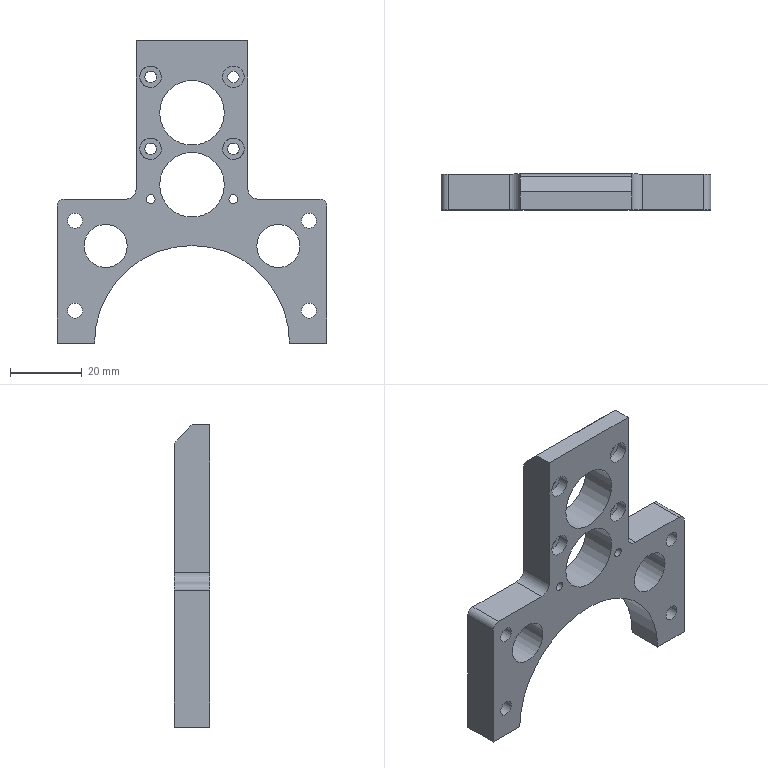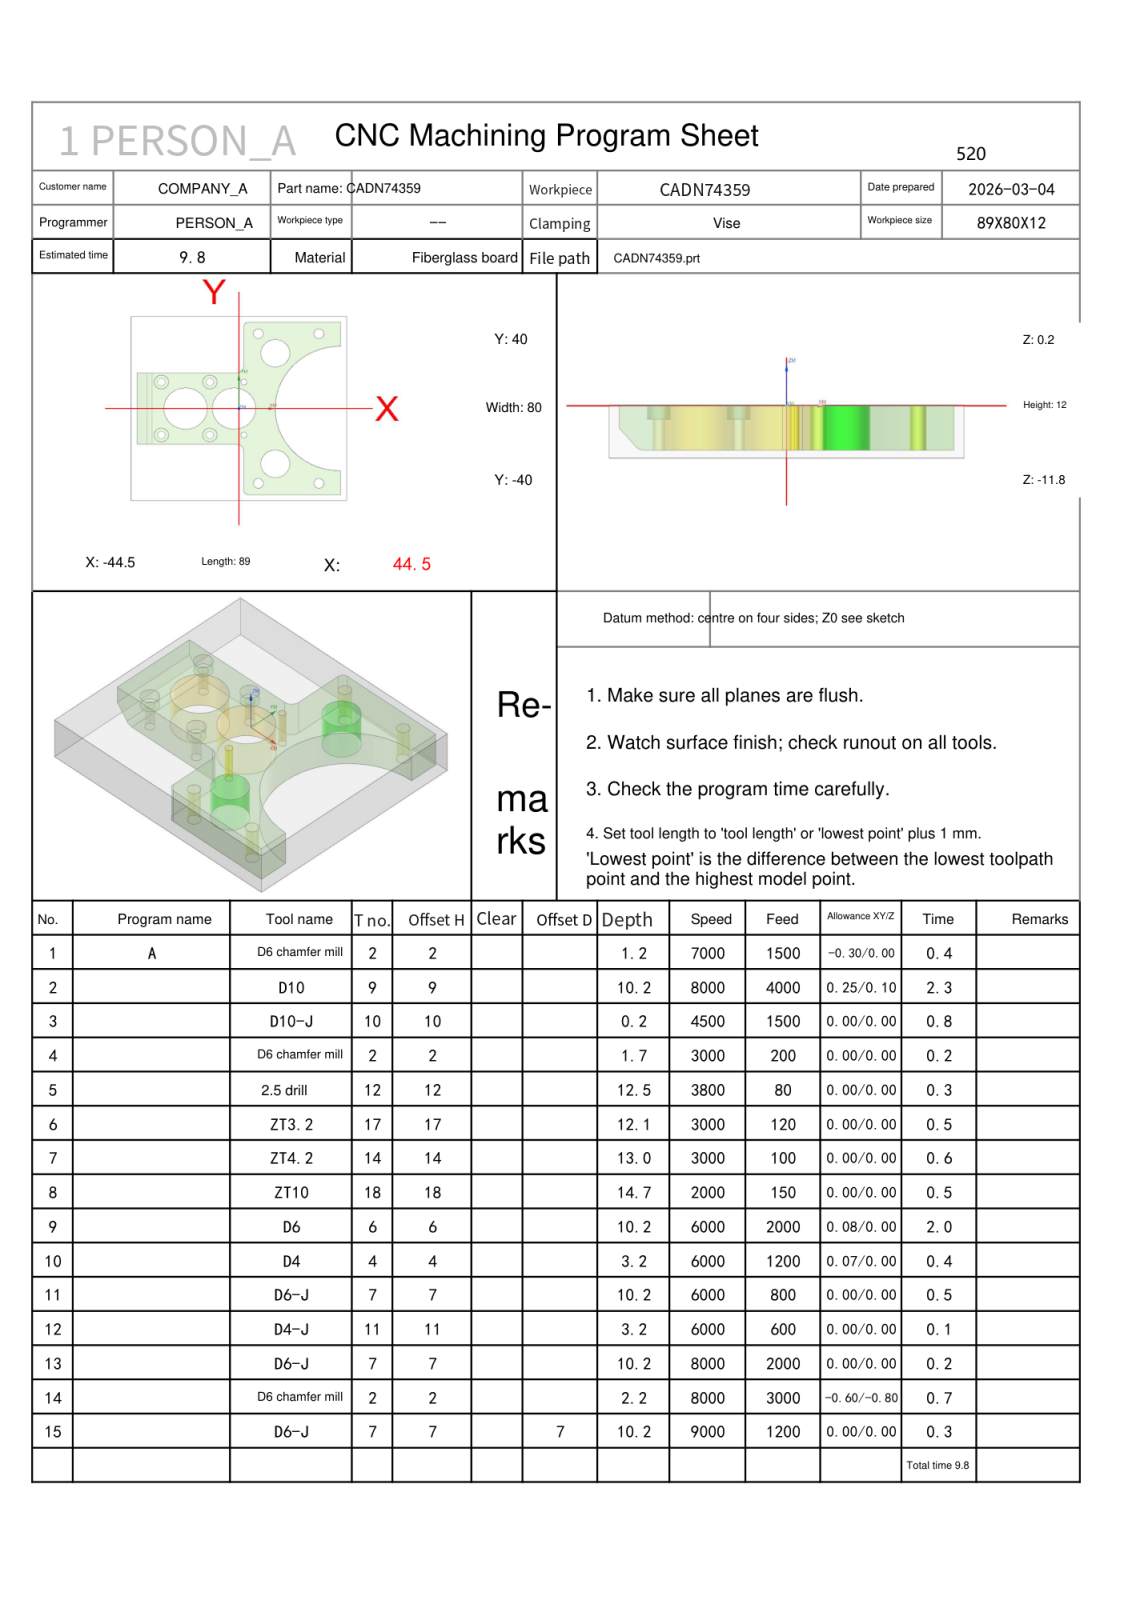NC program | NX | posted by the shop | part box 75 x 10 x 84 mm
Lines 2990 to 4435 of 4435:
N13 T07 M06
(D6-J  D=6. R=0. H=07 ce=0.00 di=0.00)
G00 G90 G54 X-1.603 Y-22.103 M03 S8000
G43 H07 Z50.
M08
Z.1
G01 X-1.596 Y-22.101 Z.009 F2000.
X-1.574 Y-22.096 Z-.073
X-1.541 Y-22.087 Z-.147
X-1.497 Y-22.073 Z-.212
X-1.447 Y-22.054 Z-.269
X-1.391 Y-22.03 Z-.319
X-1.332 Y-22. Z-.361
X-1.272 Y-21.964 Z-.397
X-1.212 Y-21.922 Z-.427
X-1.156 Y-21.872 Z-.451
X-1.106 Y-21.815 Z-.47
X-1.063 Y-21.75 Z-.484
X-1.029 Y-21.676 Z-.493
X-1.008 Y-21.594 Z-.498
X-1. Y-21.503 Z-.5
Y-18.512
Y-18.5
X-4.003
X-4.072 Y-18.516 Z-.502
X-4.117 Y-18.562 Z-.506
X-4.139 Y-18.635 Z-.513
X-4.141 Y-18.731 Z-.522
X-4.123 Y-18.847 Z-.534
X-4.088 Y-18.979 Z-.547
X-4.038 Y-19.124 Z-.563
X-3.974 Y-19.278 Z-.579
X-3.897 Y-19.439 Z-.597
X-3.811 Y-19.601 Z-.616
X-3.716 Y-19.763 Z-.635
X-3.482 Y-20.105 Z-.68
X-3.218 Y-20.424 Z-.727
X-2.925 Y-20.716 Z-.773
X-2.607 Y-20.981 Z-.82
X-2.265 Y-21.215 Z-.865
X-2.103 Y-21.31 Z-.884
X-1.94 Y-21.397 Z-.903
X-1.779 Y-21.473 Z-.921
X-1.625 Y-21.537 Z-.937
X-1.48 Y-21.588 Z-.953
X-1.348 Y-21.623 Z-.966
X-1.232 Y-21.641 Z-.978
X-1.135 Y-21.639 Z-.987
X-1.063 Y-21.617 Z-.994
X-1.016 Y-21.572 Z-.998
X-1. Y-21.503 Z-1.
Y-18.5
X-4.003
X-4.072 Y-18.516 Z-1.002
X-4.117 Y-18.562 Z-1.006
X-4.139 Y-18.635 Z-1.013
X-4.141 Y-18.731 Z-1.022
X-4.123 Y-18.847 Z-1.034
X-4.088 Y-18.979 Z-1.047
X-4.038 Y-19.124 Z-1.063
X-3.974 Y-19.278 Z-1.079
X-3.897 Y-19.439 Z-1.097
X-3.811 Y-19.601 Z-1.116
X-3.716 Y-19.763 Z-1.135
X-3.482 Y-20.105 Z-1.18
X-3.218 Y-20.424 Z-1.227
X-2.925 Y-20.716 Z-1.273
X-2.607 Y-20.981 Z-1.32
X-2.265 Y-21.215 Z-1.365
X-2.103 Y-21.31 Z-1.384
X-1.94 Y-21.397 Z-1.403
X-1.779 Y-21.473 Z-1.421
X-1.625 Y-21.537 Z-1.437
X-1.48 Y-21.588 Z-1.453
X-1.348 Y-21.623 Z-1.466
X-1.232 Y-21.641 Z-1.478
X-1.135 Y-21.639 Z-1.487
X-1.063 Y-21.617 Z-1.494
X-1.016 Y-21.572 Z-1.498
X-1. Y-21.503 Z-1.5
Y-18.5
X-4.003
X-4.072 Y-18.516 Z-1.502
X-4.117 Y-18.562 Z-1.506
X-4.139 Y-18.635 Z-1.513
X-4.141 Y-18.731 Z-1.522
X-4.123 Y-18.847 Z-1.534
X-4.088 Y-18.979 Z-1.547
X-4.038 Y-19.124 Z-1.563
X-3.974 Y-19.278 Z-1.579
X-3.897 Y-19.439 Z-1.597
X-3.811 Y-19.601 Z-1.616
X-3.716 Y-19.763 Z-1.635
X-3.482 Y-20.105 Z-1.68
X-3.218 Y-20.424 Z-1.727
X-2.925 Y-20.716 Z-1.773
X-2.607 Y-20.981 Z-1.82
X-2.265 Y-21.215 Z-1.865
X-2.103 Y-21.31 Z-1.884
X-1.94 Y-21.397 Z-1.903
X-1.779 Y-21.473 Z-1.921
X-1.625 Y-21.537 Z-1.937
X-1.48 Y-21.588 Z-1.953
X-1.348 Y-21.623 Z-1.966
X-1.232 Y-21.641 Z-1.978
X-1.135 Y-21.639 Z-1.987
X-1.063 Y-21.617 Z-1.994
X-1.016 Y-21.572 Z-1.998
X-1. Y-21.503 Z-2.
Y-18.5
X-4.003
X-4.072 Y-18.516 Z-2.002
X-4.117 Y-18.562 Z-2.006
X-4.139 Y-18.635 Z-2.013
X-4.141 Y-18.731 Z-2.022
X-4.123 Y-18.847 Z-2.034
X-4.088 Y-18.979 Z-2.047
X-4.038 Y-19.124 Z-2.063
X-3.974 Y-19.278 Z-2.079
X-3.897 Y-19.439 Z-2.097
X-3.811 Y-19.601 Z-2.116
X-3.716 Y-19.763 Z-2.135
X-3.482 Y-20.105 Z-2.18
X-3.218 Y-20.424 Z-2.227
X-2.925 Y-20.716 Z-2.273
X-2.607 Y-20.981 Z-2.32
X-2.265 Y-21.215 Z-2.365
X-2.103 Y-21.31 Z-2.384
X-1.94 Y-21.397 Z-2.403
X-1.779 Y-21.473 Z-2.421
X-1.625 Y-21.537 Z-2.437
X-1.48 Y-21.588 Z-2.453
X-1.348 Y-21.623 Z-2.466
X-1.232 Y-21.641 Z-2.478
X-1.135 Y-21.639 Z-2.487
X-1.063 Y-21.617 Z-2.494
X-1.016 Y-21.572 Z-2.498
X-1. Y-21.503 Z-2.5
Y-18.5
X-4.003
X-4.072 Y-18.516 Z-2.502
X-4.117 Y-18.562 Z-2.506
X-4.139 Y-18.635 Z-2.513
X-4.141 Y-18.731 Z-2.522
X-4.123 Y-18.847 Z-2.534
X-4.088 Y-18.979 Z-2.547
X-4.038 Y-19.124 Z-2.563
X-3.974 Y-19.278 Z-2.579
X-3.897 Y-19.439 Z-2.597
X-3.811 Y-19.601 Z-2.616
X-3.716 Y-19.763 Z-2.635
X-3.482 Y-20.105 Z-2.68
X-3.218 Y-20.424 Z-2.727
X-2.925 Y-20.716 Z-2.773
X-2.607 Y-20.981 Z-2.82
X-2.265 Y-21.215 Z-2.865
X-2.103 Y-21.31 Z-2.884
X-1.94 Y-21.397 Z-2.903
X-1.779 Y-21.473 Z-2.921
X-1.625 Y-21.537 Z-2.937
X-1.48 Y-21.588 Z-2.953
X-1.348 Y-21.623 Z-2.966
X-1.232 Y-21.641 Z-2.978
X-1.135 Y-21.639 Z-2.987
X-1.063 Y-21.617 Z-2.994
X-1.016 Y-21.572 Z-2.998
X-1. Y-21.503 Z-3.
Y-18.5
X-4.003
X-4.072 Y-18.516 Z-3.002
X-4.117 Y-18.562 Z-3.006
X-4.139 Y-18.635 Z-3.013
X-4.141 Y-18.731 Z-3.022
X-4.123 Y-18.847 Z-3.034
X-4.088 Y-18.979 Z-3.047
X-4.038 Y-19.124 Z-3.063
X-3.974 Y-19.278 Z-3.079
X-3.897 Y-19.439 Z-3.097
X-3.811 Y-19.601 Z-3.116
X-3.716 Y-19.763 Z-3.135
X-3.482 Y-20.105 Z-3.18
X-3.218 Y-20.424 Z-3.227
X-2.925 Y-20.716 Z-3.273
X-2.607 Y-20.981 Z-3.32
X-2.265 Y-21.215 Z-3.365
X-2.103 Y-21.31 Z-3.384
X-1.94 Y-21.397 Z-3.403
X-1.779 Y-21.473 Z-3.421
X-1.625 Y-21.537 Z-3.437
X-1.48 Y-21.588 Z-3.453
X-1.348 Y-21.623 Z-3.466
X-1.232 Y-21.641 Z-3.478
X-1.135 Y-21.639 Z-3.487
X-1.063 Y-21.617 Z-3.494
X-1.016 Y-21.572 Z-3.498
X-1. Y-21.503 Z-3.5
Y-18.5
X-4.003
X-4.072 Y-18.516 Z-3.502
X-4.117 Y-18.562 Z-3.506
X-4.139 Y-18.635 Z-3.513
X-4.141 Y-18.731 Z-3.522
X-4.123 Y-18.847 Z-3.534
X-4.088 Y-18.979 Z-3.547
X-4.038 Y-19.124 Z-3.563
X-3.974 Y-19.278 Z-3.579
X-3.897 Y-19.439 Z-3.597
X-3.811 Y-19.601 Z-3.616
X-3.716 Y-19.763 Z-3.635
X-3.482 Y-20.105 Z-3.68
X-3.218 Y-20.424 Z-3.727
X-2.925 Y-20.716 Z-3.773
X-2.607 Y-20.981 Z-3.82
X-2.265 Y-21.215 Z-3.865
X-2.103 Y-21.31 Z-3.884
X-1.94 Y-21.397 Z-3.903
X-1.779 Y-21.473 Z-3.921
X-1.625 Y-21.537 Z-3.937
X-1.48 Y-21.588 Z-3.953
X-1.348 Y-21.623 Z-3.966
X-1.232 Y-21.641 Z-3.978
X-1.135 Y-21.639 Z-3.987
X-1.063 Y-21.617 Z-3.994
X-1.016 Y-21.572 Z-3.998
X-1. Y-21.503 Z-4.
Y-18.5
X-4.003
X-4.072 Y-18.516 Z-4.002
X-4.117 Y-18.562 Z-4.006
X-4.139 Y-18.635 Z-4.013
X-4.141 Y-18.731 Z-4.022
X-4.123 Y-18.847 Z-4.034
X-4.088 Y-18.979 Z-4.047
X-4.038 Y-19.124 Z-4.063
X-3.974 Y-19.278 Z-4.079
X-3.897 Y-19.439 Z-4.097
X-3.811 Y-19.601 Z-4.116
X-3.716 Y-19.763 Z-4.135
X-3.482 Y-20.105 Z-4.18
X-3.218 Y-20.424 Z-4.227
X-2.925 Y-20.716 Z-4.273
X-2.607 Y-20.981 Z-4.32
X-2.265 Y-21.215 Z-4.365
X-2.103 Y-21.31 Z-4.384
X-1.94 Y-21.397 Z-4.403
X-1.779 Y-21.473 Z-4.421
X-1.625 Y-21.537 Z-4.437
X-1.48 Y-21.588 Z-4.453
X-1.348 Y-21.623 Z-4.466
X-1.232 Y-21.641 Z-4.478
X-1.135 Y-21.639 Z-4.487
X-1.063 Y-21.617 Z-4.494
X-1.016 Y-21.572 Z-4.498
X-1. Y-21.503 Z-4.5
Y-18.5
X-4.003
X-4.072 Y-18.516 Z-4.502
X-4.117 Y-18.562 Z-4.506
X-4.139 Y-18.635 Z-4.513
X-4.141 Y-18.731 Z-4.522
X-4.123 Y-18.847 Z-4.534
X-4.088 Y-18.979 Z-4.547
X-4.038 Y-19.124 Z-4.563
X-3.974 Y-19.278 Z-4.579
X-3.897 Y-19.439 Z-4.597
X-3.811 Y-19.601 Z-4.616
X-3.716 Y-19.763 Z-4.635
X-3.482 Y-20.105 Z-4.68
X-3.218 Y-20.424 Z-4.727
X-2.925 Y-20.716 Z-4.773
X-2.607 Y-20.981 Z-4.82
X-2.265 Y-21.215 Z-4.865
X-2.103 Y-21.31 Z-4.884
X-1.94 Y-21.397 Z-4.903
X-1.779 Y-21.473 Z-4.921
X-1.625 Y-21.537 Z-4.937
X-1.48 Y-21.588 Z-4.953
X-1.348 Y-21.623 Z-4.966
X-1.232 Y-21.641 Z-4.978
X-1.135 Y-21.639 Z-4.987
X-1.063 Y-21.617 Z-4.994
X-1.016 Y-21.572 Z-4.998
X-1. Y-21.503 Z-5.
Y-18.5
X-4.003
X-4.072 Y-18.516 Z-5.002
X-4.117 Y-18.562 Z-5.006
X-4.139 Y-18.635 Z-5.013
X-4.141 Y-18.731 Z-5.022
X-4.123 Y-18.847 Z-5.034
X-4.088 Y-18.979 Z-5.047
X-4.038 Y-19.124 Z-5.063
X-3.974 Y-19.278 Z-5.079
X-3.897 Y-19.439 Z-5.097
X-3.811 Y-19.601 Z-5.116
X-3.716 Y-19.763 Z-5.135
X-3.482 Y-20.105 Z-5.18
X-3.218 Y-20.424 Z-5.227
X-2.925 Y-20.716 Z-5.273
X-2.607 Y-20.981 Z-5.32
X-2.265 Y-21.215 Z-5.365
X-2.103 Y-21.31 Z-5.384
X-1.94 Y-21.397 Z-5.403
X-1.779 Y-21.473 Z-5.421
X-1.625 Y-21.537 Z-5.437
X-1.48 Y-21.588 Z-5.453
X-1.348 Y-21.623 Z-5.466
X-1.232 Y-21.641 Z-5.478
X-1.135 Y-21.639 Z-5.487
X-1.063 Y-21.617 Z-5.494
X-1.016 Y-21.572 Z-5.498
X-1. Y-21.503 Z-5.5
Y-18.5
X-4.003
X-4.072 Y-18.516 Z-5.502
X-4.117 Y-18.562 Z-5.506
X-4.139 Y-18.635 Z-5.513
X-4.141 Y-18.731 Z-5.522
X-4.123 Y-18.847 Z-5.534
X-4.088 Y-18.979 Z-5.547
X-4.038 Y-19.124 Z-5.563
X-3.974 Y-19.278 Z-5.579
X-3.897 Y-19.439 Z-5.597
X-3.811 Y-19.601 Z-5.616
X-3.716 Y-19.763 Z-5.635
X-3.482 Y-20.105 Z-5.68
X-3.218 Y-20.424 Z-5.727
X-2.925 Y-20.716 Z-5.773
X-2.607 Y-20.981 Z-5.82
X-2.265 Y-21.215 Z-5.865
X-2.103 Y-21.31 Z-5.884
X-1.94 Y-21.397 Z-5.903
X-1.779 Y-21.473 Z-5.921
X-1.625 Y-21.537 Z-5.937
X-1.48 Y-21.588 Z-5.953
X-1.348 Y-21.623 Z-5.966
X-1.232 Y-21.641 Z-5.978
X-1.135 Y-21.639 Z-5.987
X-1.063 Y-21.617 Z-5.994
X-1.016 Y-21.572 Z-5.998
X-1. Y-21.503 Z-6.
Y-18.5
X-4.003
X-4.072 Y-18.516 Z-6.002
X-4.117 Y-18.562 Z-6.006
X-4.139 Y-18.635 Z-6.013
X-4.141 Y-18.731 Z-6.022
X-4.123 Y-18.847 Z-6.034
X-4.088 Y-18.979 Z-6.047
X-4.038 Y-19.124 Z-6.063
X-3.974 Y-19.278 Z-6.079
X-3.897 Y-19.439 Z-6.097
X-3.811 Y-19.601 Z-6.116
X-3.716 Y-19.763 Z-6.135
X-3.482 Y-20.105 Z-6.18
X-3.218 Y-20.424 Z-6.227
X-2.925 Y-20.716 Z-6.273
X-2.607 Y-20.981 Z-6.32
X-2.265 Y-21.215 Z-6.365
X-2.103 Y-21.31 Z-6.384
X-1.94 Y-21.397 Z-6.403
X-1.779 Y-21.473 Z-6.421
X-1.625 Y-21.537 Z-6.437
X-1.48 Y-21.588 Z-6.453
X-1.348 Y-21.623 Z-6.466
X-1.232 Y-21.641 Z-6.478
X-1.135 Y-21.639 Z-6.487
X-1.063 Y-21.617 Z-6.494
X-1.016 Y-21.572 Z-6.498
X-1. Y-21.503 Z-6.5
Y-18.5
X-4.003
X-4.072 Y-18.516 Z-6.502
X-4.117 Y-18.562 Z-6.506
X-4.139 Y-18.635 Z-6.513
X-4.141 Y-18.731 Z-6.522
X-4.123 Y-18.847 Z-6.534
X-4.088 Y-18.979 Z-6.547
X-4.038 Y-19.124 Z-6.563
X-3.974 Y-19.278 Z-6.579
X-3.897 Y-19.439 Z-6.597
X-3.811 Y-19.601 Z-6.616
X-3.716 Y-19.763 Z-6.635
X-3.482 Y-20.105 Z-6.68
X-3.218 Y-20.424 Z-6.727
X-2.925 Y-20.716 Z-6.773
X-2.607 Y-20.981 Z-6.82
X-2.265 Y-21.215 Z-6.865
X-2.103 Y-21.31 Z-6.884
X-1.94 Y-21.397 Z-6.903
X-1.779 Y-21.473 Z-6.921
X-1.625 Y-21.537 Z-6.937
X-1.48 Y-21.588 Z-6.953
X-1.348 Y-21.623 Z-6.966
X-1.232 Y-21.641 Z-6.978
X-1.135 Y-21.639 Z-6.987
X-1.063 Y-21.617 Z-6.994
X-1.016 Y-21.572 Z-6.998
X-1. Y-21.503 Z-7.
Y-18.5
X-4.003
X-4.072 Y-18.516 Z-7.002
X-4.117 Y-18.562 Z-7.006
X-4.139 Y-18.635 Z-7.013
X-4.141 Y-18.731 Z-7.022
X-4.123 Y-18.847 Z-7.034
X-4.088 Y-18.979 Z-7.047
X-4.038 Y-19.124 Z-7.063
X-3.974 Y-19.278 Z-7.079
X-3.897 Y-19.439 Z-7.097
X-3.811 Y-19.601 Z-7.116
X-3.716 Y-19.763 Z-7.135
X-3.482 Y-20.105 Z-7.18
X-3.218 Y-20.424 Z-7.227
X-2.925 Y-20.716 Z-7.273
X-2.607 Y-20.981 Z-7.32
X-2.265 Y-21.215 Z-7.365
X-2.103 Y-21.31 Z-7.384
X-1.94 Y-21.397 Z-7.403
X-1.779 Y-21.473 Z-7.421
X-1.625 Y-21.537 Z-7.437
X-1.48 Y-21.588 Z-7.453
X-1.348 Y-21.623 Z-7.466
X-1.232 Y-21.641 Z-7.478
X-1.135 Y-21.639 Z-7.487
X-1.063 Y-21.617 Z-7.494
X-1.016 Y-21.572 Z-7.498
X-1. Y-21.503 Z-7.5
Y-18.5
X-4.003
X-4.072 Y-18.516 Z-7.502
X-4.117 Y-18.562 Z-7.506
X-4.139 Y-18.635 Z-7.513
X-4.141 Y-18.731 Z-7.522
X-4.123 Y-18.847 Z-7.534
X-4.088 Y-18.979 Z-7.547
X-4.038 Y-19.124 Z-7.563
X-3.974 Y-19.278 Z-7.579
X-3.897 Y-19.439 Z-7.597
X-3.811 Y-19.601 Z-7.616
X-3.716 Y-19.763 Z-7.635
X-3.482 Y-20.105 Z-7.68
X-3.218 Y-20.424 Z-7.727
X-2.925 Y-20.716 Z-7.773
X-2.607 Y-20.981 Z-7.82
X-2.265 Y-21.215 Z-7.865
X-2.103 Y-21.31 Z-7.884
X-1.94 Y-21.397 Z-7.903
X-1.779 Y-21.473 Z-7.921
X-1.625 Y-21.537 Z-7.937
X-1.48 Y-21.588 Z-7.953
X-1.348 Y-21.623 Z-7.966
X-1.232 Y-21.641 Z-7.978
X-1.135 Y-21.639 Z-7.987
X-1.063 Y-21.617 Z-7.994
X-1.016 Y-21.572 Z-7.998
X-1. Y-21.503 Z-8.
Y-18.5
X-4.003
X-4.072 Y-18.516 Z-8.002
X-4.117 Y-18.562 Z-8.006
X-4.139 Y-18.635 Z-8.013
X-4.141 Y-18.731 Z-8.022
X-4.123 Y-18.847 Z-8.034
X-4.088 Y-18.979 Z-8.047
X-4.038 Y-19.124 Z-8.063
X-3.974 Y-19.278 Z-8.079
X-3.897 Y-19.439 Z-8.097
X-3.811 Y-19.601 Z-8.116
X-3.716 Y-19.763 Z-8.135
X-3.482 Y-20.105 Z-8.18
X-3.218 Y-20.424 Z-8.227
X-2.925 Y-20.716 Z-8.273
X-2.607 Y-20.981 Z-8.32
X-2.265 Y-21.215 Z-8.365
X-2.103 Y-21.31 Z-8.384
X-1.94 Y-21.397 Z-8.403
X-1.779 Y-21.473 Z-8.421
X-1.625 Y-21.537 Z-8.437
X-1.48 Y-21.588 Z-8.453
X-1.348 Y-21.623 Z-8.466
X-1.232 Y-21.641 Z-8.478
X-1.135 Y-21.639 Z-8.487
X-1.063 Y-21.617 Z-8.494
X-1.016 Y-21.572 Z-8.498
X-1. Y-21.503 Z-8.5
Y-18.5
X-4.003
X-4.072 Y-18.516 Z-8.502
X-4.117 Y-18.562 Z-8.506
X-4.139 Y-18.635 Z-8.513
X-4.141 Y-18.731 Z-8.522
X-4.123 Y-18.847 Z-8.534
X-4.088 Y-18.979 Z-8.547
X-4.038 Y-19.124 Z-8.563
X-3.974 Y-19.278 Z-8.579
X-3.897 Y-19.439 Z-8.597
X-3.811 Y-19.601 Z-8.616
X-3.716 Y-19.763 Z-8.635
X-3.482 Y-20.105 Z-8.68
X-3.218 Y-20.424 Z-8.727
X-2.925 Y-20.716 Z-8.773
X-2.607 Y-20.981 Z-8.82
X-2.265 Y-21.215 Z-8.865
X-2.103 Y-21.31 Z-8.884
X-1.94 Y-21.397 Z-8.903
X-1.779 Y-21.473 Z-8.921
X-1.625 Y-21.537 Z-8.937
X-1.48 Y-21.588 Z-8.953
X-1.348 Y-21.623 Z-8.966
X-1.232 Y-21.641 Z-8.978
X-1.135 Y-21.639 Z-8.987
X-1.063 Y-21.617 Z-8.994
X-1.016 Y-21.572 Z-8.998
X-1. Y-21.503 Z-9.
Y-18.5
X-4.003
X-4.072 Y-18.516 Z-9.002
X-4.117 Y-18.562 Z-9.006
X-4.139 Y-18.635 Z-9.013
X-4.141 Y-18.731 Z-9.022
X-4.123 Y-18.847 Z-9.034
X-4.088 Y-18.979 Z-9.047
X-4.038 Y-19.124 Z-9.063
X-3.974 Y-19.278 Z-9.079
X-3.897 Y-19.439 Z-9.097
X-3.811 Y-19.601 Z-9.116
X-3.716 Y-19.763 Z-9.135
X-3.482 Y-20.105 Z-9.18
X-3.218 Y-20.424 Z-9.227
X-2.925 Y-20.716 Z-9.273
X-2.607 Y-20.981 Z-9.32
X-2.265 Y-21.215 Z-9.365
X-2.103 Y-21.31 Z-9.384
X-1.94 Y-21.397 Z-9.403
X-1.779 Y-21.473 Z-9.421
X-1.625 Y-21.537 Z-9.437
X-1.48 Y-21.588 Z-9.453
X-1.348 Y-21.623 Z-9.466
X-1.232 Y-21.641 Z-9.478
X-1.135 Y-21.639 Z-9.487
X-1.063 Y-21.617 Z-9.494
X-1.016 Y-21.572 Z-9.498
X-1. Y-21.503 Z-9.5
Y-18.5
X-4.003
X-4.072 Y-18.516 Z-9.502
X-4.117 Y-18.562 Z-9.506
X-4.139 Y-18.635 Z-9.513
X-4.141 Y-18.731 Z-9.522
X-4.123 Y-18.847 Z-9.534
X-4.088 Y-18.979 Z-9.547
X-4.038 Y-19.124 Z-9.563
X-3.974 Y-19.278 Z-9.579
X-3.897 Y-19.439 Z-9.597
X-3.811 Y-19.601 Z-9.616
X-3.716 Y-19.763 Z-9.635
X-3.482 Y-20.105 Z-9.68
X-3.218 Y-20.424 Z-9.727
X-2.925 Y-20.716 Z-9.773
X-2.607 Y-20.981 Z-9.82
X-2.265 Y-21.215 Z-9.865
X-2.103 Y-21.31 Z-9.884
X-1.94 Y-21.397 Z-9.903
X-1.779 Y-21.473 Z-9.921
X-1.625 Y-21.537 Z-9.937
X-1.48 Y-21.588 Z-9.953
X-1.348 Y-21.623 Z-9.966
X-1.232 Y-21.641 Z-9.978
X-1.135 Y-21.639 Z-9.987
X-1.063 Y-21.617 Z-9.994
X-1.016 Y-21.572 Z-9.998
X-1. Y-21.503 Z-10.
Y-18.5
X-4.003
X-4.094 Y-18.508 Z-9.998
X-4.176 Y-18.529 Z-9.993
X-4.25 Y-18.562 Z-9.984
X-4.315 Y-18.605 Z-9.97
X-4.372 Y-18.656 Z-9.951
X-4.422 Y-18.711 Z-9.927
X-4.464 Y-18.77 Z-9.897
X-4.5 Y-18.83 Z-9.861
X-4.53 Y-18.889 Z-9.819
X-4.554 Y-18.944 Z-9.769
X-4.573 Y-18.995 Z-9.712
X-4.587 Y-19.038 Z-9.647
X-4.596 Y-19.071 Z-9.573
X-4.601 Y-19.092 Z-9.491
X-4.603 Y-19.1 Z-9.4
G00 Z50.
Y19.103
Z.1
G01 X-4.602 Y19.096 Z.009
X-4.596 Y19.074 Z-.073
X-4.587 Y19.041 Z-.147
X-4.573 Y18.998 Z-.212
X-4.554 Y18.947 Z-.269
X-4.53 Y18.891 Z-.319
X-4.5 Y18.832 Z-.361
X-4.464 Y18.772 Z-.397
X-4.422 Y18.712 Z-.427
X-4.372 Y18.656 Z-.451
X-4.315 Y18.606 Z-.47
X-4.25 Y18.563 Z-.484
X-4.176 Y18.529 Z-.493
X-4.094 Y18.508 Z-.498
X-4.003 Y18.5 Z-.5
X-1.01
X-1.
Y21.503
X-1.016 Y21.572 Z-.502
X-1.062 Y21.617 Z-.506
X-1.135 Y21.639 Z-.513
X-1.231 Y21.641 Z-.522
X-1.347 Y21.623 Z-.534
X-1.479 Y21.588 Z-.547
X-1.624 Y21.538 Z-.563
X-1.778 Y21.474 Z-.579
X-1.939 Y21.397 Z-.597
X-2.101 Y21.311 Z-.616
X-2.263 Y21.216 Z-.635
X-2.605 Y20.982 Z-.68
X-2.924 Y20.718 Z-.727
X-3.216 Y20.425 Z-.773
X-3.481 Y20.107 Z-.82
X-3.715 Y19.765 Z-.865
X-3.81 Y19.603 Z-.884
X-3.897 Y19.44 Z-.903
X-3.973 Y19.279 Z-.921
X-4.037 Y19.125 Z-.937
X-4.088 Y18.98 Z-.953
X-4.123 Y18.848 Z-.966
X-4.141 Y18.732 Z-.978
X-4.139 Y18.635 Z-.987
X-4.117 Y18.563 Z-.994
X-4.072 Y18.516 Z-.998
X-4.003 Y18.5 Z-1.
X-1.
Y21.503
X-1.016 Y21.572 Z-1.002
X-1.062 Y21.617 Z-1.006
X-1.135 Y21.639 Z-1.013
X-1.231 Y21.641 Z-1.022
X-1.347 Y21.623 Z-1.034
X-1.479 Y21.588 Z-1.047
X-1.624 Y21.538 Z-1.063
X-1.778 Y21.474 Z-1.079
X-1.939 Y21.397 Z-1.097
X-2.101 Y21.311 Z-1.116
X-2.263 Y21.216 Z-1.135
X-2.605 Y20.982 Z-1.18
X-2.924 Y20.718 Z-1.227
X-3.216 Y20.425 Z-1.273
X-3.481 Y20.107 Z-1.32
X-3.715 Y19.765 Z-1.365
X-3.81 Y19.603 Z-1.384
X-3.897 Y19.44 Z-1.403
X-3.973 Y19.279 Z-1.421
X-4.037 Y19.125 Z-1.437
X-4.088 Y18.98 Z-1.453
X-4.123 Y18.848 Z-1.466
X-4.141 Y18.732 Z-1.478
X-4.139 Y18.635 Z-1.487
X-4.117 Y18.563 Z-1.494
X-4.072 Y18.516 Z-1.498
X-4.003 Y18.5 Z-1.5
X-1.
Y21.503
X-1.016 Y21.572 Z-1.502
X-1.062 Y21.617 Z-1.506
X-1.135 Y21.639 Z-1.513
X-1.231 Y21.641 Z-1.522
X-1.347 Y21.623 Z-1.534
X-1.479 Y21.588 Z-1.547
X-1.624 Y21.538 Z-1.563
X-1.778 Y21.474 Z-1.579
X-1.939 Y21.397 Z-1.597
X-2.101 Y21.311 Z-1.616
X-2.263 Y21.216 Z-1.635
X-2.605 Y20.982 Z-1.68
X-2.924 Y20.718 Z-1.727
X-3.216 Y20.425 Z-1.773
X-3.481 Y20.107 Z-1.82
X-3.715 Y19.765 Z-1.865
X-3.81 Y19.603 Z-1.884
X-3.897 Y19.44 Z-1.903
X-3.973 Y19.279 Z-1.921
X-4.037 Y19.125 Z-1.937
X-4.088 Y18.98 Z-1.953
X-4.123 Y18.848 Z-1.966
X-4.141 Y18.732 Z-1.978
X-4.139 Y18.635 Z-1.987
X-4.117 Y18.563 Z-1.994
X-4.072 Y18.516 Z-1.998
X-4.003 Y18.5 Z-2.
X-1.
Y21.503
X-1.016 Y21.572 Z-2.002
X-1.062 Y21.617 Z-2.006
X-1.135 Y21.639 Z-2.013
X-1.231 Y21.641 Z-2.022
X-1.347 Y21.623 Z-2.034
X-1.479 Y21.588 Z-2.047
X-1.624 Y21.538 Z-2.063
X-1.778 Y21.474 Z-2.079
X-1.939 Y21.397 Z-2.097
X-2.101 Y21.311 Z-2.116
X-2.263 Y21.216 Z-2.135
X-2.605 Y20.982 Z-2.18
X-2.924 Y20.718 Z-2.227
X-3.216 Y20.425 Z-2.273
X-3.481 Y20.107 Z-2.32
X-3.715 Y19.765 Z-2.365
X-3.81 Y19.603 Z-2.384
X-3.897 Y19.44 Z-2.403
X-3.973 Y19.279 Z-2.421
X-4.037 Y19.125 Z-2.437
X-4.088 Y18.98 Z-2.453
X-4.123 Y18.848 Z-2.466
X-4.141 Y18.732 Z-2.478
X-4.139 Y18.635 Z-2.487
X-4.117 Y18.563 Z-2.494
X-4.072 Y18.516 Z-2.498
X-4.003 Y18.5 Z-2.5
X-1.
Y21.503
X-1.016 Y21.572 Z-2.502
X-1.062 Y21.617 Z-2.506
X-1.135 Y21.639 Z-2.513
X-1.231 Y21.641 Z-2.522
X-1.347 Y21.623 Z-2.534
X-1.479 Y21.588 Z-2.547
X-1.624 Y21.538 Z-2.563
X-1.778 Y21.474 Z-2.579
X-1.939 Y21.397 Z-2.597
X-2.101 Y21.311 Z-2.616
X-2.263 Y21.216 Z-2.635
X-2.605 Y20.982 Z-2.68
X-2.924 Y20.718 Z-2.727
X-3.216 Y20.425 Z-2.773
X-3.481 Y20.107 Z-2.82
X-3.715 Y19.765 Z-2.865
X-3.81 Y19.603 Z-2.884
X-3.897 Y19.44 Z-2.903
X-3.973 Y19.279 Z-2.921
X-4.037 Y19.125 Z-2.937
X-4.088 Y18.98 Z-2.953
X-4.123 Y18.848 Z-2.966
X-4.141 Y18.732 Z-2.978
X-4.139 Y18.635 Z-2.987
X-4.117 Y18.563 Z-2.994
X-4.072 Y18.516 Z-2.998
X-4.003 Y18.5 Z-3.
X-1.
Y21.503
X-1.016 Y21.572 Z-3.002
X-1.062 Y21.617 Z-3.006
X-1.135 Y21.639 Z-3.013
X-1.231 Y21.641 Z-3.022
X-1.347 Y21.623 Z-3.034
X-1.479 Y21.588 Z-3.047
X-1.624 Y21.538 Z-3.063
X-1.778 Y21.474 Z-3.079
X-1.939 Y21.397 Z-3.097
X-2.101 Y21.311 Z-3.116
X-2.263 Y21.216 Z-3.135
X-2.605 Y20.982 Z-3.18
X-2.924 Y20.718 Z-3.227
X-3.216 Y20.425 Z-3.273
X-3.481 Y20.107 Z-3.32
X-3.715 Y19.765 Z-3.365
X-3.81 Y19.603 Z-3.384
X-3.897 Y19.44 Z-3.403
X-3.973 Y19.279 Z-3.421
X-4.037 Y19.125 Z-3.437
X-4.088 Y18.98 Z-3.453
X-4.123 Y18.848 Z-3.466
X-4.141 Y18.732 Z-3.478
X-4.139 Y18.635 Z-3.487
X-4.117 Y18.563 Z-3.494
X-4.072 Y18.516 Z-3.498
X-4.003 Y18.5 Z-3.5
X-1.
Y21.503
X-1.016 Y21.572 Z-3.502
X-1.062 Y21.617 Z-3.506
X-1.135 Y21.639 Z-3.513
X-1.231 Y21.641 Z-3.522
X-1.347 Y21.623 Z-3.534
X-1.479 Y21.588 Z-3.547
X-1.624 Y21.538 Z-3.563
X-1.778 Y21.474 Z-3.579
X-1.939 Y21.397 Z-3.597
X-2.101 Y21.311 Z-3.616
X-2.263 Y21.216 Z-3.635
X-2.605 Y20.982 Z-3.68
X-2.924 Y20.718 Z-3.727
X-3.216 Y20.425 Z-3.773
X-3.481 Y20.107 Z-3.82
X-3.715 Y19.765 Z-3.865
X-3.81 Y19.603 Z-3.884
X-3.897 Y19.44 Z-3.903
X-3.973 Y19.279 Z-3.921
X-4.037 Y19.125 Z-3.937
X-4.088 Y18.98 Z-3.953
X-4.123 Y18.848 Z-3.966
X-4.141 Y18.732 Z-3.978
X-4.139 Y18.635 Z-3.987
X-4.117 Y18.563 Z-3.994
X-4.072 Y18.516 Z-3.998
X-4.003 Y18.5 Z-4.
X-1.
Y21.503
X-1.016 Y21.572 Z-4.002
X-1.062 Y21.617 Z-4.006
X-1.135 Y21.639 Z-4.013
X-1.231 Y21.641 Z-4.022
X-1.347 Y21.623 Z-4.034
X-1.479 Y21.588 Z-4.047
X-1.624 Y21.538 Z-4.063
X-1.778 Y21.474 Z-4.079
X-1.939 Y21.397 Z-4.097
X-2.101 Y21.311 Z-4.116
X-2.263 Y21.216 Z-4.135
X-2.605 Y20.982 Z-4.18
X-2.924 Y20.718 Z-4.227
X-3.216 Y20.425 Z-4.273
X-3.481 Y20.107 Z-4.32
X-3.715 Y19.765 Z-4.365
X-3.81 Y19.603 Z-4.384
X-3.897 Y19.44 Z-4.403
X-3.973 Y19.279 Z-4.421
X-4.037 Y19.125 Z-4.437
X-4.088 Y18.98 Z-4.453
X-4.123 Y18.848 Z-4.466
X-4.141 Y18.732 Z-4.478
X-4.139 Y18.635 Z-4.487
X-4.117 Y18.563 Z-4.494
X-4.072 Y18.516 Z-4.498
X-4.003 Y18.5 Z-4.5
X-1.
Y21.503
X-1.016 Y21.572 Z-4.502
X-1.062 Y21.617 Z-4.506
X-1.135 Y21.639 Z-4.513
X-1.231 Y21.641 Z-4.522
X-1.347 Y21.623 Z-4.534
X-1.479 Y21.588 Z-4.547
X-1.624 Y21.538 Z-4.563
X-1.778 Y21.474 Z-4.579
X-1.939 Y21.397 Z-4.597
X-2.101 Y21.311 Z-4.616
X-2.263 Y21.216 Z-4.635
X-2.605 Y20.982 Z-4.68
X-2.924 Y20.718 Z-4.727
X-3.216 Y20.425 Z-4.773
X-3.481 Y20.107 Z-4.82
X-3.715 Y19.765 Z-4.865
X-3.81 Y19.603 Z-4.884
X-3.897 Y19.44 Z-4.903
X-3.973 Y19.279 Z-4.921
X-4.037 Y19.125 Z-4.937
X-4.088 Y18.98 Z-4.953
X-4.123 Y18.848 Z-4.966
X-4.141 Y18.732 Z-4.978
X-4.139 Y18.635 Z-4.987
X-4.117 Y18.563 Z-4.994
X-4.072 Y18.516 Z-4.998
X-4.003 Y18.5 Z-5.
X-1.
Y21.503
X-1.016 Y21.572 Z-5.002
X-1.062 Y21.617 Z-5.006
X-1.135 Y21.639 Z-5.013
X-1.231 Y21.641 Z-5.022
X-1.347 Y21.623 Z-5.034
X-1.479 Y21.588 Z-5.047
X-1.624 Y21.538 Z-5.063
X-1.778 Y21.474 Z-5.079
X-1.939 Y21.397 Z-5.097
X-2.101 Y21.311 Z-5.116
X-2.263 Y21.216 Z-5.135
X-2.605 Y20.982 Z-5.18
X-2.924 Y20.718 Z-5.227
X-3.216 Y20.425 Z-5.273
X-3.481 Y20.107 Z-5.32
X-3.715 Y19.765 Z-5.365
X-3.81 Y19.603 Z-5.384
X-3.897 Y19.44 Z-5.403
X-3.973 Y19.279 Z-5.421
X-4.037 Y19.125 Z-5.437
X-4.088 Y18.98 Z-5.453
X-4.123 Y18.848 Z-5.466
X-4.141 Y18.732 Z-5.478
X-4.139 Y18.635 Z-5.487
X-4.117 Y18.563 Z-5.494
X-4.072 Y18.516 Z-5.498
X-4.003 Y18.5 Z-5.5
X-1.
Y21.503
X-1.016 Y21.572 Z-5.502
X-1.062 Y21.617 Z-5.506
X-1.135 Y21.639 Z-5.513
X-1.231 Y21.641 Z-5.522
X-1.347 Y21.623 Z-5.534
X-1.479 Y21.588 Z-5.547
X-1.624 Y21.538 Z-5.563
X-1.778 Y21.474 Z-5.579
X-1.939 Y21.397 Z-5.597
X-2.101 Y21.311 Z-5.616
X-2.263 Y21.216 Z-5.635
X-2.605 Y20.982 Z-5.68
X-2.924 Y20.718 Z-5.727
X-3.216 Y20.425 Z-5.773
X-3.481 Y20.107 Z-5.82
X-3.715 Y19.765 Z-5.865
X-3.81 Y19.603 Z-5.884
X-3.897 Y19.44 Z-5.903
X-3.973 Y19.279 Z-5.921
X-4.037 Y19.125 Z-5.937
X-4.088 Y18.98 Z-5.953
X-4.123 Y18.848 Z-5.966
X-4.141 Y18.732 Z-5.978
X-4.139 Y18.635 Z-5.987
X-4.117 Y18.563 Z-5.994
X-4.072 Y18.516 Z-5.998
X-4.003 Y18.5 Z-6.
X-1.
Y21.503
X-1.016 Y21.572 Z-6.002
X-1.062 Y21.617 Z-6.006
X-1.135 Y21.639 Z-6.013
X-1.231 Y21.641 Z-6.022
X-1.347 Y21.623 Z-6.034
X-1.479 Y21.588 Z-6.047
X-1.624 Y21.538 Z-6.063
X-1.778 Y21.474 Z-6.079
X-1.939 Y21.397 Z-6.097
X-2.101 Y21.311 Z-6.116
X-2.263 Y21.216 Z-6.135
X-2.605 Y20.982 Z-6.18
X-2.924 Y20.718 Z-6.227
X-3.216 Y20.425 Z-6.273
X-3.481 Y20.107 Z-6.32
X-3.715 Y19.765 Z-6.365
X-3.81 Y19.603 Z-6.384
X-3.897 Y19.44 Z-6.403
X-3.973 Y19.279 Z-6.421
X-4.037 Y19.125 Z-6.437
X-4.088 Y18.98 Z-6.453
X-4.123 Y18.848 Z-6.466
X-4.141 Y18.732 Z-6.478
X-4.139 Y18.635 Z-6.487
X-4.117 Y18.563 Z-6.494
X-4.072 Y18.516 Z-6.498
X-4.003 Y18.5 Z-6.5
X-1.
Y21.503
X-1.016 Y21.572 Z-6.502
X-1.062 Y21.617 Z-6.506
X-1.135 Y21.639 Z-6.513
X-1.231 Y21.641 Z-6.522
X-1.347 Y21.623 Z-6.534
X-1.479 Y21.588 Z-6.547
X-1.624 Y21.538 Z-6.563
X-1.778 Y21.474 Z-6.579
X-1.939 Y21.397 Z-6.597
X-2.101 Y21.311 Z-6.616
X-2.263 Y21.216 Z-6.635
X-2.605 Y20.982 Z-6.68
X-2.924 Y20.718 Z-6.727
X-3.216 Y20.425 Z-6.773
X-3.481 Y20.107 Z-6.82
X-3.715 Y19.765 Z-6.865
X-3.81 Y19.603 Z-6.884
X-3.897 Y19.44 Z-6.903
X-3.973 Y19.279 Z-6.921
X-4.037 Y19.125 Z-6.937
X-4.088 Y18.98 Z-6.953
X-4.123 Y18.848 Z-6.966
X-4.141 Y18.732 Z-6.978
X-4.139 Y18.635 Z-6.987
X-4.117 Y18.563 Z-6.994
X-4.072 Y18.516 Z-6.998
X-4.003 Y18.5 Z-7.
X-1.
Y21.503
X-1.016 Y21.572 Z-7.002
X-1.062 Y21.617 Z-7.006
X-1.135 Y21.639 Z-7.013
X-1.231 Y21.641 Z-7.022
X-1.347 Y21.623 Z-7.034
X-1.479 Y21.588 Z-7.047
X-1.624 Y21.538 Z-7.063
X-1.778 Y21.474 Z-7.079
X-1.939 Y21.397 Z-7.097
X-2.101 Y21.311 Z-7.116
X-2.263 Y21.216 Z-7.135
X-2.605 Y20.982 Z-7.18
X-2.924 Y20.718 Z-7.227
X-3.216 Y20.425 Z-7.273
X-3.481 Y20.107 Z-7.32
X-3.715 Y19.765 Z-7.365
X-3.81 Y19.603 Z-7.384
X-3.897 Y19.44 Z-7.403
X-3.973 Y19.279 Z-7.421
X-4.037 Y19.125 Z-7.437
X-4.088 Y18.98 Z-7.453
X-4.123 Y18.848 Z-7.466
X-4.141 Y18.732 Z-7.478
X-4.139 Y18.635 Z-7.487
X-4.117 Y18.563 Z-7.494
X-4.072 Y18.516 Z-7.498
X-4.003 Y18.5 Z-7.5
X-1.
Y21.503
X-1.016 Y21.572 Z-7.502
X-1.062 Y21.617 Z-7.506
X-1.135 Y21.639 Z-7.513
X-1.231 Y21.641 Z-7.522
X-1.347 Y21.623 Z-7.534
X-1.479 Y21.588 Z-7.547
X-1.624 Y21.538 Z-7.563
X-1.778 Y21.474 Z-7.579
X-1.939 Y21.397 Z-7.597
X-2.101 Y21.311 Z-7.616
X-2.263 Y21.216 Z-7.635
X-2.605 Y20.982 Z-7.68
X-2.924 Y20.718 Z-7.727
X-3.216 Y20.425 Z-7.773
X-3.481 Y20.107 Z-7.82
X-3.715 Y19.765 Z-7.865
X-3.81 Y19.603 Z-7.884
X-3.897 Y19.44 Z-7.903
X-3.973 Y19.279 Z-7.921
X-4.037 Y19.125 Z-7.937
X-4.088 Y18.98 Z-7.953
X-4.123 Y18.848 Z-7.966
X-4.141 Y18.732 Z-7.978
X-4.139 Y18.635 Z-7.987
X-4.117 Y18.563 Z-7.994
X-4.072 Y18.516 Z-7.998
X-4.003 Y18.5 Z-8.
X-1.
Y21.503
X-1.016 Y21.572 Z-8.002
X-1.062 Y21.617 Z-8.006
X-1.135 Y21.639 Z-8.013
X-1.231 Y21.641 Z-8.022
X-1.347 Y21.623 Z-8.034
X-1.479 Y21.588 Z-8.047
X-1.624 Y21.538 Z-8.063
X-1.778 Y21.474 Z-8.079
X-1.939 Y21.397 Z-8.097
X-2.101 Y21.311 Z-8.116
X-2.263 Y21.216 Z-8.135
X-2.605 Y20.982 Z-8.18
X-2.924 Y20.718 Z-8.227
X-3.216 Y20.425 Z-8.273
X-3.481 Y20.107 Z-8.32
X-3.715 Y19.765 Z-8.365
X-3.81 Y19.603 Z-8.384
X-3.897 Y19.44 Z-8.403
X-3.973 Y19.279 Z-8.421
X-4.037 Y19.125 Z-8.437
X-4.088 Y18.98 Z-8.453
X-4.123 Y18.848 Z-8.466
X-4.141 Y18.732 Z-8.478
X-4.139 Y18.635 Z-8.487
X-4.117 Y18.563 Z-8.494
X-4.072 Y18.516 Z-8.498
X-4.003 Y18.5 Z-8.5
X-1.
Y21.503
X-1.016 Y21.572 Z-8.502
X-1.062 Y21.617 Z-8.506
X-1.135 Y21.639 Z-8.513
X-1.231 Y21.641 Z-8.522
X-1.347 Y21.623 Z-8.534
X-1.479 Y21.588 Z-8.547
X-1.624 Y21.538 Z-8.563
X-1.778 Y21.474 Z-8.579
X-1.939 Y21.397 Z-8.597
X-2.101 Y21.311 Z-8.616
X-2.263 Y21.216 Z-8.635
X-2.605 Y20.982 Z-8.68
X-2.924 Y20.718 Z-8.727
X-3.216 Y20.425 Z-8.773
X-3.481 Y20.107 Z-8.82
X-3.715 Y19.765 Z-8.865
X-3.81 Y19.603 Z-8.884
X-3.897 Y19.44 Z-8.903
X-3.973 Y19.279 Z-8.921
X-4.037 Y19.125 Z-8.937
X-4.088 Y18.98 Z-8.953
X-4.123 Y18.848 Z-8.966
X-4.141 Y18.732 Z-8.978
X-4.139 Y18.635 Z-8.987
X-4.117 Y18.563 Z-8.994
X-4.072 Y18.516 Z-8.998
X-4.003 Y18.5 Z-9.
X-1.
Y21.503
X-1.016 Y21.572 Z-9.002
X-1.062 Y21.617 Z-9.006
X-1.135 Y21.639 Z-9.013
X-1.231 Y21.641 Z-9.022
X-1.347 Y21.623 Z-9.034
X-1.479 Y21.588 Z-9.047
X-1.624 Y21.538 Z-9.063
X-1.778 Y21.474 Z-9.079
X-1.939 Y21.397 Z-9.097
X-2.101 Y21.311 Z-9.116
X-2.263 Y21.216 Z-9.135
X-2.605 Y20.982 Z-9.18
X-2.924 Y20.718 Z-9.227
X-3.216 Y20.425 Z-9.273
X-3.481 Y20.107 Z-9.32
X-3.715 Y19.765 Z-9.365
X-3.81 Y19.603 Z-9.384
X-3.897 Y19.44 Z-9.403
X-3.973 Y19.279 Z-9.421
X-4.037 Y19.125 Z-9.437
X-4.088 Y18.98 Z-9.453
X-4.123 Y18.848 Z-9.466
X-4.141 Y18.732 Z-9.478
X-4.139 Y18.635 Z-9.487
X-4.117 Y18.563 Z-9.494
X-4.072 Y18.516 Z-9.498
X-4.003 Y18.5 Z-9.5
X-1.
Y21.503
X-1.016 Y21.572 Z-9.502
X-1.062 Y21.617 Z-9.506
X-1.135 Y21.639 Z-9.513
X-1.231 Y21.641 Z-9.522
X-1.347 Y21.623 Z-9.534
X-1.479 Y21.588 Z-9.547
X-1.624 Y21.538 Z-9.563
X-1.778 Y21.474 Z-9.579
X-1.939 Y21.397 Z-9.597
X-2.101 Y21.311 Z-9.616
X-2.263 Y21.216 Z-9.635
X-2.605 Y20.982 Z-9.68
X-2.924 Y20.718 Z-9.727
X-3.216 Y20.425 Z-9.773
X-3.481 Y20.107 Z-9.82
X-3.715 Y19.765 Z-9.865
X-3.81 Y19.603 Z-9.884
X-3.897 Y19.44 Z-9.903
X-3.973 Y19.279 Z-9.921
X-4.037 Y19.125 Z-9.937
X-4.088 Y18.98 Z-9.953
X-4.123 Y18.848 Z-9.966
X-4.141 Y18.732 Z-9.978
X-4.139 Y18.635 Z-9.987
X-4.117 Y18.563 Z-9.994
X-4.072 Y18.516 Z-9.998
X-4.003 Y18.5 Z-10.
X-1.
Y21.503
X-1.008 Y21.594 Z-9.998
X-1.029 Y21.676 Z-9.993
X-1.062 Y21.75 Z-9.984
X-1.105 Y21.815 Z-9.97
X-1.156 Y21.872 Z-9.951
X-1.211 Y21.922 Z-9.927
X-1.27 Y21.964 Z-9.897
X-1.33 Y22. Z-9.861
X-1.389 Y22.03 Z-9.819
X-1.444 Y22.054 Z-9.769
X-1.495 Y22.073 Z-9.712
X-1.538 Y22.087 Z-9.647
X-1.571 Y22.096 Z-9.573
X-1.592 Y22.101 Z-9.491
X-1.6 Y22.103 Z-9.4
G00 Z50.
G91 G28 Z0.0
M05
M09
G91 G28 Z0.0
M01
N14 T02 M06
(D6 chamfer mill  D=6. R=0. H=02 ce=0.00 di=0.00)
G00 G90 G54 X-21.75 Y17.628 M03 S8000
G43 H02 Z50.
M08
Z2.099
G01 Z-1.5 F3000.
G03 X-21.83 Y17.328 I.52 J-.3
X-21.53 Y16.808 I.6 J0.0
G01 X-21.5 Y16.8
X-1.
G03 X.7 Y18.5 I0.0 J1.7
G01 Y35.5
G02 X4. Y38.8 I3.3 J0.0
G01 X42.
G02 X43.3 Y37.5 I0.0 J-1.3
G01 Y27.1
G02 X42. Y25.8 I-1.3 J0.0
G03 X16.2 Y0.0 I0.0 J-25.8
X42. Y-25.8 I25.8 J0.0
G02 X43.3 Y-27.1 I0.0 J-1.3
G01 Y-37.5
G02 X42. Y-38.8 I-1.3 J0.0
G01 X4.
G02 X.7 Y-35.5 I0.0 J3.3
G01 Y-18.5
G03 X-1. Y-16.8 I-1.7 J0.0
G01 X-42.
G02 X-43.3 Y-15.5 I0.0 J1.3
G01 Y15.5
G02 X-42. Y16.8 I1.3 J0.0
G01 X-21.5
X-21.47 Y16.808
G03 X-21.17 Y17.328 I-.3 J.52
X-21.25 Y17.628 I-.6 J0.0
G01 Z2.099
G00 Z50.
X4.885 Y-.289
Z2.127
G01 Z-1.5
G03 X5.16 Y-.355 I.275 J.533
X5.693 Y-.03 I0.0 J.6
G01 X5.7 Y0.0
G03 X-2. Y7.7 I-7.7 J0.0
X-9.7 Y0.0 I0.0 J-7.7
X-2. Y-7.7 I7.7 J0.0
X5.7 Y0.0 I0.0 J7.7
G01 X5.693 Y.03
G03 X5.16 Y.355 I-.533 J-.275
X4.885 Y.289 I0.0 J-.6
G01 Z2.125
G00 Z50.
X-15.115 Y-.289
Z2.127
G01 Z-1.5
G03 X-14.84 Y-.355 I.275 J.533
X-14.307 Y-.03 I0.0 J.6
G01 X-14.3 Y0.0
G03 X-22. Y7.7 I-7.7 J0.0
X-29.7 Y0.0 I0.0 J-7.7
X-22. Y-7.7 I7.7 J0.0
X-14.3 Y0.0 I0.0 J7.7
G01 X-14.307 Y.03
G03 X-14.84 Y.355 I-.533 J-.275
X-15.115 Y.289 I0.0 J-.6
G01 Z2.125
G00 Z50.
G00 G90 X2. Y11.5 M03 S5000
Z50.
G98 G81 X2. Y11.5 Z-1.75 R3. F150.
Y-11.5
G80
G00 Z50.
G00 G90 X7.848 Y32.87 M03 S6000
Z50.
Z-.8
G01 Z-1.3 F600.
X7.684 Y32.879
X7.6 Y32.882
G03 X6.6 Y32.5 I0.0 J-1.5
X8. Y31.1 I1.4 J0.0
X9.4 Y32.5 I0.0 J1.4
X8. Y33.9 I-1.4 J0.0
X6.6 Y32.5 I0.0 J-1.4
X7.6 Y32.118 I1. J1.118
G01 X7.684 Y32.121
X7.848 Y32.13
Z-.8
G00 Z50.
X32.848 Y32.87
Z-.8
G01 Z-1.3
X32.684 Y32.879
X32.6 Y32.882
G03 X31.6 Y32.5 I0.0 J-1.5
X33. Y31.1 I1.4 J0.0
X34.4 Y32.5 I0.0 J1.4
X33. Y33.9 I-1.4 J0.0
X31.6 Y32.5 I0.0 J-1.4
X32.6 Y32.118 I1. J1.118
G01 X32.684 Y32.121
X32.848 Y32.13
Z-.8
G00 Z50.
Y-32.13
Z-.8
G01 Z-1.3
X32.684 Y-32.121
X32.6 Y-32.118
G03 X31.6 Y-32.5 I0.0 J-1.5
X33. Y-33.9 I1.4 J0.0
X34.4 Y-32.5 I0.0 J1.4
X33. Y-31.1 I-1.4 J0.0
X31.6 Y-32.5 I0.0 J-1.4
X32.6 Y-32.882 I1. J1.118
G01 X32.684 Y-32.879
X32.848 Y-32.87
Z-.8
G00 Z50.
X7.848 Y-32.13
Z-.8
G01 Z-1.3
X7.684 Y-32.121
X7.6 Y-32.118
G03 X6.6 Y-32.5 I0.0 J-1.5
X8. Y-33.9 I1.4 J0.0
X9.4 Y-32.5 I0.0 J1.4
X8. Y-31.1 I-1.4 J0.0
X6.6 Y-32.5 I0.0 J-1.4
X7.6 Y-32.882 I1. J1.118
G01 X7.684 Y-32.879
X7.848 Y-32.87
Z-.8
G00 Z50.
G00 G90 X-32.066 Y-11.207 M03 S6000
Z50.
Z-1.5
G01 Z-2. F600.
X-32.194 Y-11.192
X-32.375 Y-11.181
G03 X-33.3 Y-11.5 I0.0 J-1.5
X-32. Y-12.8 I1.3 J0.0
X-30.7 Y-11.5 I0.0 J1.3
X-32. Y-10.2 I-1.3 J0.0
X-33.3 Y-11.5 I0.0 J-1.3
X-32.375 Y-11.819 I.925 J1.181
G01 X-32.194 Y-11.808
X-32.066 Y-11.793
Z-1.5
G00 Z50.
X-12.066 Y-11.207
Z-1.5
G01 Z-2.
X-12.194 Y-11.192
X-12.375 Y-11.181
G03 X-13.3 Y-11.5 I0.0 J-1.5
X-12. Y-12.8 I1.3 J0.0
X-10.7 Y-11.5 I0.0 J1.3
X-12. Y-10.2 I-1.3 J0.0
X-13.3 Y-11.5 I0.0 J-1.3
X-12.375 Y-11.819 I.925 J1.181
G01 X-12.194 Y-11.808
X-12.066 Y-11.793
Z-1.5
G00 Z50.
X-11.934 Y11.207
Z-1.5
G01 Z-2.
X-11.806 Y11.192
X-11.625 Y11.181
G03 X-10.7 Y11.5 I0.0 J1.5
X-12. Y12.8 I-1.3 J0.0
X-13.3 Y11.5 I0.0 J-1.3
X-12. Y10.2 I1.3 J0.0
X-10.7 Y11.5 I0.0 J1.3
X-11.625 Y11.819 I-.925 J-1.181
G01 X-11.806 Y11.808
X-11.934 Y11.793
Z-1.5
G00 Z50.
X-31.934 Y11.207
Z-1.5
G01 Z-2.
X-31.806 Y11.192
X-31.625 Y11.181
G03 X-30.7 Y11.5 I0.0 J1.5
X-32. Y12.8 I-1.3 J0.0
X-33.3 Y11.5 I0.0 J-1.3
X-32. Y10.2 I1.3 J0.0
X-30.7 Y11.5 I0.0 J1.3
X-31.625 Y11.819 I-.925 J-1.181
G01 X-31.806 Y11.808
X-31.934 Y11.793
Z-1.5
G00 Z50.
G00 G90 X16.8 Y-27. M03 S6000
Z50.
Z-1.
G01 Z-1.5 F600.
G03 X19.8 Y-24. I0.0 J3.
X15. Y-19.2 I-4.8 J0.0
X10.2 Y-24. I0.0 J-4.8
X15. Y-28.8 I4.8 J0.0
X19.8 Y-24. I0.0 J4.8
X16.8 Y-21. I-3. J0.0
G01 Z-1.
G00 Z50.
Y21.
Z-1.
G01 Z-1.5
G03 X19.8 Y24. I0.0 J3.
X15. Y28.8 I-4.8 J0.0
X10.2 Y24. I0.0 J-4.8
X15. Y19.2 I4.8 J0.0
X19.8 Y24. I0.0 J4.8
X16.8 Y27. I-3. J0.0
G01 Z-1.
G00 Z50.
G91 G28 Z0.0
M05
M09
G91 G28 Z0.0
M01
N15 T07 M06
(D6-J  D=6. R=0. H=07 ce=0.00 di=0.00)
G00 G90 G54 X43.017 Y-41.573 M03 S9000
G43 H07 Z50.
M08
Z-9.5
G01 Z-10. F1200.
G41 D07
X42.992 Y-41.375
G03 X42. Y-40.5 I-.992 J-.125
G01 X4.
G02 X-1. Y-35.5 I0.0 J5.
G01 Y-18.5
X-42.
G02 X-45. Y-15.5 I0.0 J3.
G01 Y15.5
G02 X-42. Y18.5 I3. J0.0
G01 X-1.
Y35.5
G02 X4. Y40.5 I5. J0.0
G01 X42.
G02 X45. Y37.5 I0.0 J-3.
G01 Y27.1
G02 X42. Y24.1 I-3. J0.0
G03 X17.9 Y0.0 I0.0 J-24.1
X42. Y-24.1 I24.1 J0.0
G02 X45. Y-27.1 I0.0 J-3.
G01 Y-37.5
G02 X42. Y-40.5 I-3. J0.0
G01 X41.5
G03 X40.5 Y-41.5 I0.0 J-1.
G01 G40 Y-41.7
Z-9.5
G00 Z50.
M05
M09
G91 G28 Z0.0
G91 G28 Y0.0
M30
%